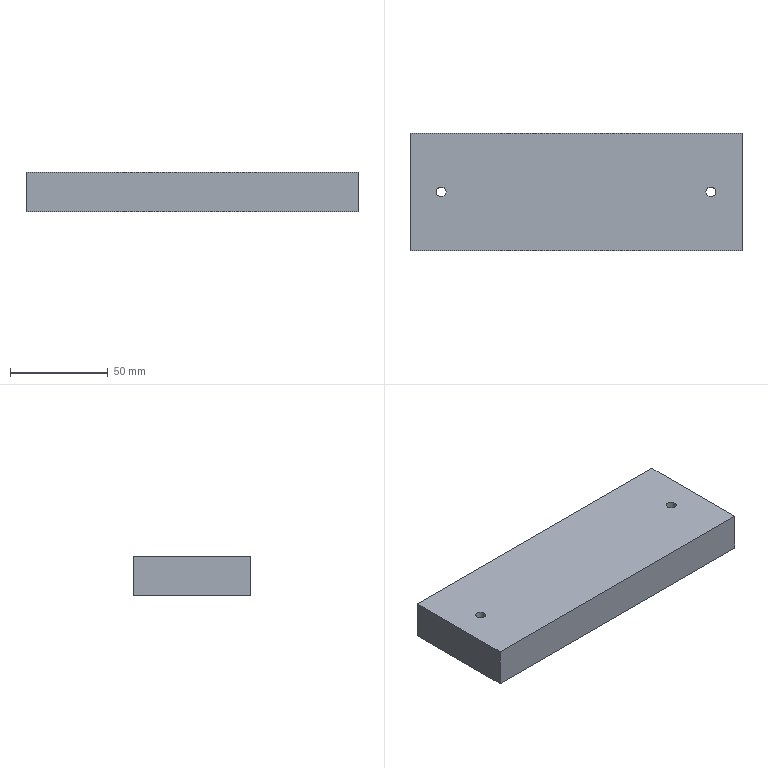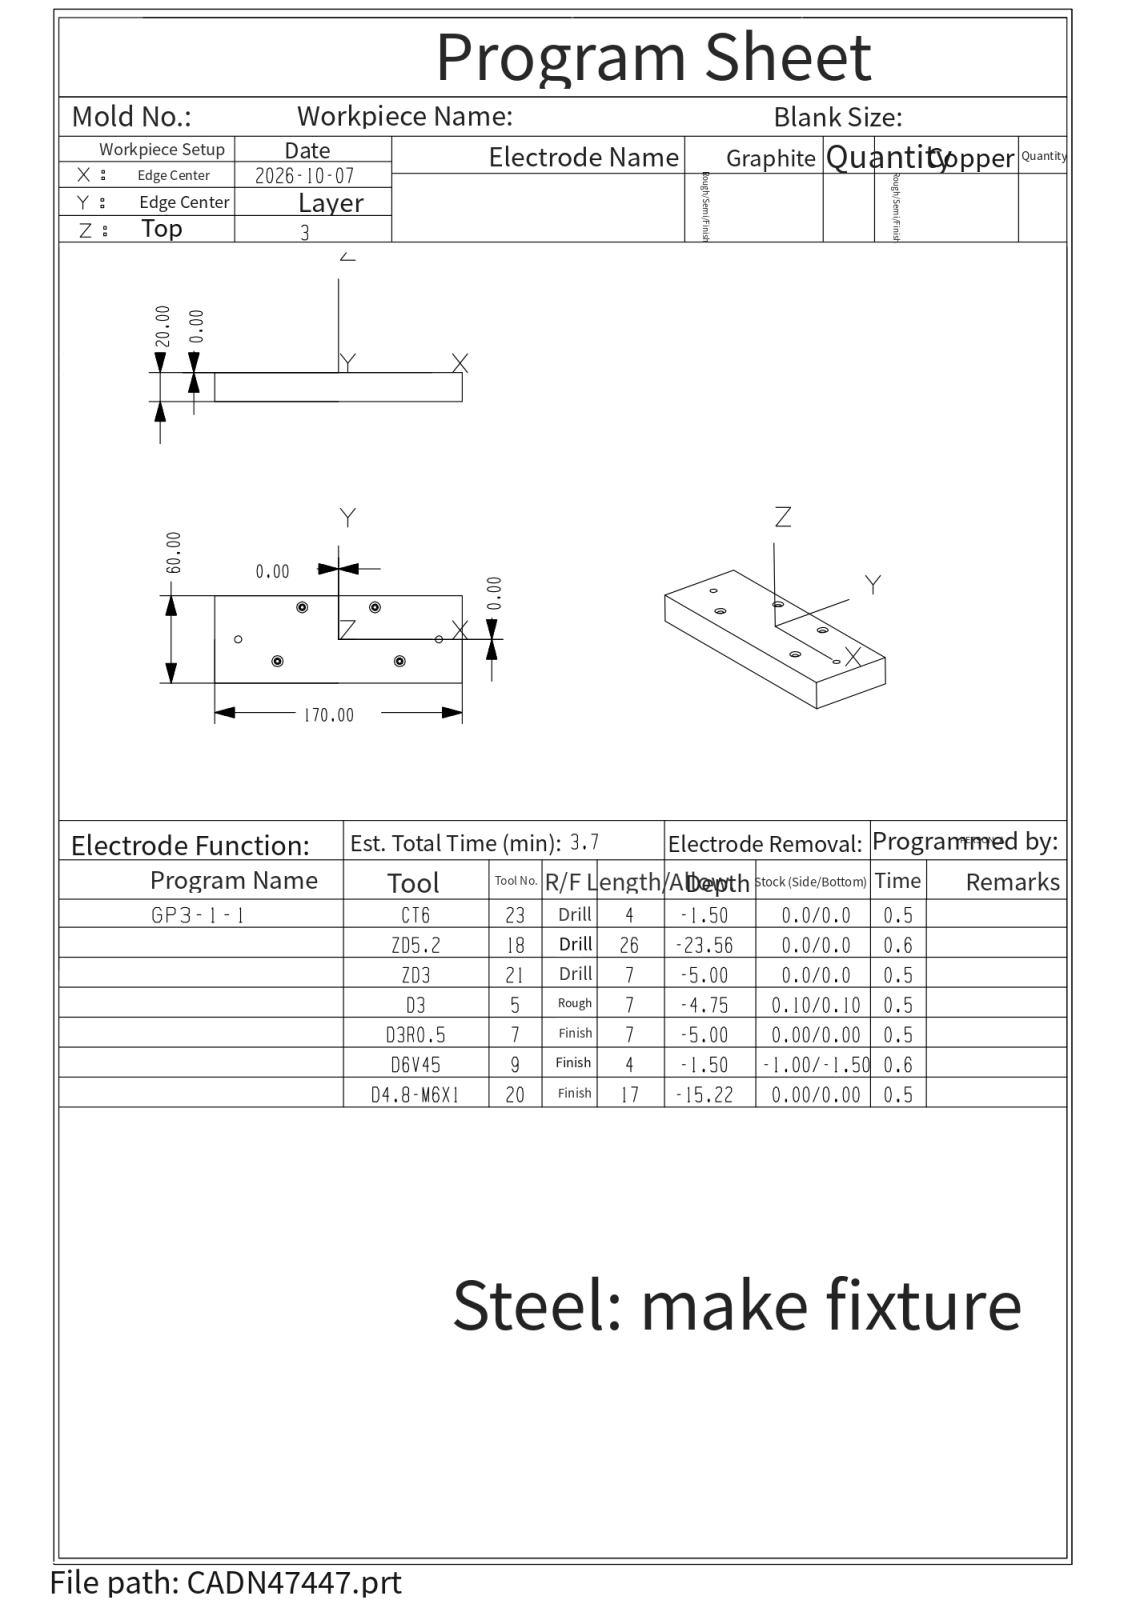NC program | NX | posted by the shop | part box 170 x 60 x 20 mm
Lines 1 to 59 of 14163:
%
O0001
G40 G49 G80 G90
G91 G28 Z0.0
N01
T23 M06
T18
( name=CT6    T=23 )
( XY = 0.00 )
( Z = 0.00 )
G00 G90 G54 X69. Y0.0 S3000 M03
G43 Z10. H23 M08
G98 G81 X69. Y0.0 Z-1.5 R1. F1000.
X42.001 Y-15.
X25.001 Y22.
X-24.999
X-41.999 Y-15.
X-69. Y0.0
G80
G00 Z10.
M05
M09
G91 G28 Z0.0
M01
N02
T18 M06
T21
( name=ZD5.2    T=18 )
( XY = 0.00 )
( Z = 0.00 )
G00 G90 G54 X69. Y0.0 S800 M03
G43 Z10. H18 M08
G98 G83 X69. Y0.0 Z-23.562 R1. F100. Q2.
X-69.
G80
G00 Z10.
M05
M09
G91 G28 Z0.0
M01
N03
T21 M06
T05
( name=ZD3    T=21 )
( XY = 0.00 )
( Z = 0.00 )
G00 G90 G54 X42.001 Y-15. S800 M03
G43 Z10. H21 M08
G98 G83 X42.001 Y-15. Z-5. R1. F100. Q2.
X25.001 Y22.
X-24.999
X-41.999 Y-15.
G80
G00 Z10.
M05
M09
G91 G28 Z0.0
M01
N04